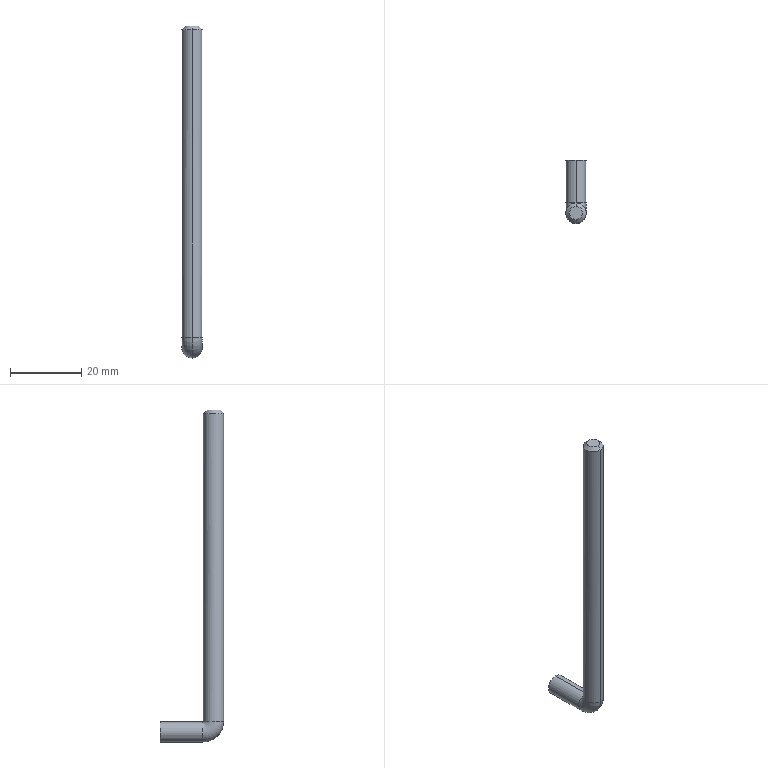Part | STEP file | RJWD-DY-0102_X2_5DE667DC95E8_37 | 1 solid | 10 faces | box 5.7 x 17.85 x 93.35 mm | volume 2651 mm3 | cylinder 4 | cone 2 | plane 2 | torus 2 | commonest cylinder face diameters 5.7 x4
STEP:
#1=CARTESIAN_POINT('',(0.,0.,0.));
#2=DIRECTION('',(0.,0.,1.));
#3=DIRECTION('',(1.,0.,0.));
#4=AXIS2_PLACEMENT_3D('',#1,#2,#3);
#5=CARTESIAN_POINT('',(-506.773,4247.223,1752.144));
#6=VERTEX_POINT('',#5);
#7=CARTESIAN_POINT('',(-503.923,4250.073,1752.144));
#8=VERTEX_POINT('',#7);
#9=CARTESIAN_POINT('',(-506.773,4250.073,1752.144));
#10=DIRECTION('',(0.,0.,1.));
#11=DIRECTION('',(0.,-1.,0.));
#12=AXIS2_PLACEMENT_3D('',#9,#10,#11);
#13=CIRCLE('',#12,2.85);
#14=CARTESIAN_POINT('',(-506.773,4250.073,1752.644));
#15=DIRECTION('',(0.,0.,-1.));
#16=DIRECTION('',(1.,0.,0.));
#17=AXIS2_PLACEMENT_3D('',#14,#15,#16);
#18=CONICAL_SURFACE('',#17,2.35,0.7854);
#19=CARTESIAN_POINT('',(1.571,0.5));
#20=DIRECTION('',(-1.,0.));
#21=VECTOR('',#20,1.);
#22=LINE('',#19,#21);
#23=(GEOMETRIC_REPRESENTATION_CONTEXT(2)PARAMETRIC_REPRESENTATION_CONTEXT()REPRESENTATION_CONTEXT('',''));
#24=DEFINITIONAL_REPRESENTATION('',(#22),#23);
#25=PCURVE('',#18,#24);
#26=CARTESIAN_POINT('',(-506.773,4250.073,1665.644));
#27=DIRECTION('',(0.,0.,1.));
#28=DIRECTION('',(0.,1.,0.));
#29=AXIS2_PLACEMENT_3D('',#26,#27,#28);
#30=CYLINDRICAL_SURFACE('',#29,2.85);
#31=CARTESIAN_POINT('',(3.142,86.5));
#32=DIRECTION('',(1.,0.));
#33=VECTOR('',#32,1.);
#34=LINE('',#31,#33);
#35=(GEOMETRIC_REPRESENTATION_CONTEXT(2)PARAMETRIC_REPRESENTATION_CONTEXT()REPRESENTATION_CONTEXT('',''));
#36=DEFINITIONAL_REPRESENTATION('',(#34),#35);
#37=PCURVE('',#30,#36);
#38=SURFACE_CURVE('',#13,(#25,#37),.PCURVE_S1.);
#39=EDGE_CURVE('',#6,#8,#38,.T.);
#40=ORIENTED_EDGE('',*,*,#39,.T.);
#41=CARTESIAN_POINT('',(-506.773,4252.923,1752.144));
#42=VERTEX_POINT('',#41);
#43=CARTESIAN_POINT('',(-506.773,4250.073,1752.144));
#44=DIRECTION('',(0.,0.,1.));
#45=DIRECTION('',(1.,0.,0.));
#46=AXIS2_PLACEMENT_3D('',#43,#44,#45);
#47=CIRCLE('',#46,2.85);
#48=CARTESIAN_POINT('',(0.,0.5));
#49=DIRECTION('',(-1.,0.));
#50=VECTOR('',#49,1.);
#51=LINE('',#48,#50);
#52=(GEOMETRIC_REPRESENTATION_CONTEXT(2)PARAMETRIC_REPRESENTATION_CONTEXT()REPRESENTATION_CONTEXT('',''));
#53=DEFINITIONAL_REPRESENTATION('',(#51),#52);
#54=PCURVE('',#18,#53);
#55=CARTESIAN_POINT('',(4.712,86.5));
#56=DIRECTION('',(1.,0.));
#57=VECTOR('',#56,1.);
#58=LINE('',#55,#57);
#59=(GEOMETRIC_REPRESENTATION_CONTEXT(2)PARAMETRIC_REPRESENTATION_CONTEXT()REPRESENTATION_CONTEXT('',''));
#60=DEFINITIONAL_REPRESENTATION('',(#58),#59);
#61=PCURVE('',#30,#60);
#62=SURFACE_CURVE('',#47,(#54,#61),.PCURVE_S1.);
#63=EDGE_CURVE('',#8,#42,#62,.T.);
#64=ORIENTED_EDGE('',*,*,#63,.T.);
#65=CARTESIAN_POINT('',(-506.773,4251.923,1753.144));
#66=VERTEX_POINT('',#65);
#67=CARTESIAN_POINT('',(-506.773,4251.923,1753.144));
#68=DIRECTION('',(0.,0.7071,-0.7071));
#69=VECTOR('',#68,1.);
#70=LINE('',#67,#69);
#71=CARTESIAN_POINT('',(-1.571,-0.5));
#72=DIRECTION('',(0.,1.));
#73=VECTOR('',#72,1.);
#74=LINE('',#71,#73);
#75=(GEOMETRIC_REPRESENTATION_CONTEXT(2)PARAMETRIC_REPRESENTATION_CONTEXT()REPRESENTATION_CONTEXT('',''));
#76=DEFINITIONAL_REPRESENTATION('',(#74),#75);
#77=PCURVE('',#18,#76);
#78=CARTESIAN_POINT('',(-506.773,4250.073,1752.644));
#79=DIRECTION('',(0.,0.,-1.));
#80=DIRECTION('',(1.,0.,0.));
#81=AXIS2_PLACEMENT_3D('',#78,#79,#80);
#82=CONICAL_SURFACE('',#81,2.35,0.7854);
#83=CARTESIAN_POINT('',(4.712,-0.5));
#84=DIRECTION('',(0.,1.));
#85=VECTOR('',#84,1.);
#86=LINE('',#83,#85);
#87=(GEOMETRIC_REPRESENTATION_CONTEXT(2)PARAMETRIC_REPRESENTATION_CONTEXT()REPRESENTATION_CONTEXT('',''));
#88=DEFINITIONAL_REPRESENTATION('',(#86),#87);
#89=PCURVE('',#82,#88);
#90=SURFACE_CURVE('',#70,(#77,#89),.PCURVE_S1.);
#91=EDGE_CURVE('',#66,#42,#90,.T.);
#92=ORIENTED_EDGE('',*,*,#91,.F.);
#93=CARTESIAN_POINT('',(-504.923,4250.073,1753.144));
#94=VERTEX_POINT('',#93);
#95=CARTESIAN_POINT('',(-506.773,4250.073,1753.144));
#96=DIRECTION('',(0.,0.,1.));
#97=DIRECTION('',(1.,0.,0.));
#98=AXIS2_PLACEMENT_3D('',#95,#96,#97);
#99=CIRCLE('',#98,1.85);
#100=CARTESIAN_POINT('',(0.,-0.5));
#101=DIRECTION('',(-1.,0.));
#102=VECTOR('',#101,1.);
#103=LINE('',#100,#102);
#104=(GEOMETRIC_REPRESENTATION_CONTEXT(2)PARAMETRIC_REPRESENTATION_CONTEXT()REPRESENTATION_CONTEXT('',''));
#105=DEFINITIONAL_REPRESENTATION('',(#103),#104);
#106=PCURVE('',#18,#105);
#107=CARTESIAN_POINT('',(-506.773,4250.073,1753.144));
#108=DIRECTION('',(0.,0.,1.));
#109=DIRECTION('',(0.,1.,0.));
#110=AXIS2_PLACEMENT_3D('',#107,#108,#109);
#111=PLANE('',#110);
#112=CARTESIAN_POINT('',(0.,0.));
#113=DIRECTION('',(0.,-1.));
#114=AXIS2_PLACEMENT_2D('',#112,#113);
#115=CIRCLE('',#114,1.85);
#116=(GEOMETRIC_REPRESENTATION_CONTEXT(2)PARAMETRIC_REPRESENTATION_CONTEXT()REPRESENTATION_CONTEXT('',''));
#117=DEFINITIONAL_REPRESENTATION('',(#115),#116);
#118=PCURVE('',#111,#117);
#119=SURFACE_CURVE('',#99,(#106,#118),.PCURVE_S1.);
#120=EDGE_CURVE('',#94,#66,#119,.T.);
#121=ORIENTED_EDGE('',*,*,#120,.F.);
#122=CARTESIAN_POINT('',(-506.773,4248.223,1753.144));
#123=VERTEX_POINT('',#122);
#124=CARTESIAN_POINT('',(-506.773,4250.073,1753.144));
#125=DIRECTION('',(0.,0.,1.));
#126=DIRECTION('',(0.,-1.,0.));
#127=AXIS2_PLACEMENT_3D('',#124,#125,#126);
#128=CIRCLE('',#127,1.85);
#129=CARTESIAN_POINT('',(1.571,-0.5));
#130=DIRECTION('',(-1.,0.));
#131=VECTOR('',#130,1.);
#132=LINE('',#129,#131);
#133=(GEOMETRIC_REPRESENTATION_CONTEXT(2)PARAMETRIC_REPRESENTATION_CONTEXT()REPRESENTATION_CONTEXT('',''));
#134=DEFINITIONAL_REPRESENTATION('',(#132),#133);
#135=PCURVE('',#18,#134);
#136=CARTESIAN_POINT('',(0.,0.));
#137=DIRECTION('',(-1.,0.));
#138=AXIS2_PLACEMENT_2D('',#136,#137);
#139=CIRCLE('',#138,1.85);
#140=(GEOMETRIC_REPRESENTATION_CONTEXT(2)PARAMETRIC_REPRESENTATION_CONTEXT()REPRESENTATION_CONTEXT('',''));
#141=DEFINITIONAL_REPRESENTATION('',(#139),#140);
#142=PCURVE('',#111,#141);
#143=SURFACE_CURVE('',#128,(#135,#142),.PCURVE_S1.);
#144=EDGE_CURVE('',#123,#94,#143,.T.);
#145=ORIENTED_EDGE('',*,*,#144,.F.);
#146=CARTESIAN_POINT('',(-506.773,4248.223,1753.144));
#147=DIRECTION('',(0.,-0.7071,-0.7071));
#148=VECTOR('',#147,1.);
#149=LINE('',#146,#148);
#150=CARTESIAN_POINT('',(1.571,-0.5));
#151=DIRECTION('',(0.,1.));
#152=VECTOR('',#151,1.);
#153=LINE('',#150,#152);
#154=(GEOMETRIC_REPRESENTATION_CONTEXT(2)PARAMETRIC_REPRESENTATION_CONTEXT()REPRESENTATION_CONTEXT('',''));
#155=DEFINITIONAL_REPRESENTATION('',(#153),#154);
#156=PCURVE('',#18,#155);
#157=CARTESIAN_POINT('',(1.571,-0.5));
#158=DIRECTION('',(0.,1.));
#159=VECTOR('',#158,1.);
#160=LINE('',#157,#159);
#161=(GEOMETRIC_REPRESENTATION_CONTEXT(2)PARAMETRIC_REPRESENTATION_CONTEXT()REPRESENTATION_CONTEXT('',''));
#162=DEFINITIONAL_REPRESENTATION('',(#160),#161);
#163=PCURVE('',#82,#162);
#164=SURFACE_CURVE('',#149,(#156,#163),.PCURVE_S1.);
#165=EDGE_CURVE('',#123,#6,#164,.T.);
#166=ORIENTED_EDGE('',*,*,#165,.T.);
#167=EDGE_LOOP('',(#40,#64,#92,#121,#145,#166));
#168=FACE_BOUND('',#167,.T.);
#169=ADVANCED_FACE('',(#168),#18,.T.);
#170=CARTESIAN_POINT('',(-509.623,4250.073,1752.144));
#171=VERTEX_POINT('',#170);
#172=CARTESIAN_POINT('',(-506.773,4250.073,1752.144));
#173=DIRECTION('',(0.,0.,1.));
#174=DIRECTION('',(0.,1.,0.));
#175=AXIS2_PLACEMENT_3D('',#172,#173,#174);
#176=CIRCLE('',#175,2.85);
#177=CARTESIAN_POINT('',(4.712,0.5));
#178=DIRECTION('',(-1.,0.));
#179=VECTOR('',#178,1.);
#180=LINE('',#177,#179);
#181=(GEOMETRIC_REPRESENTATION_CONTEXT(2)PARAMETRIC_REPRESENTATION_CONTEXT()REPRESENTATION_CONTEXT('',''));
#182=DEFINITIONAL_REPRESENTATION('',(#180),#181);
#183=PCURVE('',#82,#182);
#184=CARTESIAN_POINT('',(-506.773,4250.073,1665.644));
#185=DIRECTION('',(0.,0.,1.));
#186=DIRECTION('',(0.,1.,0.));
#187=AXIS2_PLACEMENT_3D('',#184,#185,#186);
#188=CYLINDRICAL_SURFACE('',#187,2.85);
#189=CARTESIAN_POINT('',(0.,86.5));
#190=DIRECTION('',(1.,0.));
#191=VECTOR('',#190,1.);
#192=LINE('',#189,#191);
#193=(GEOMETRIC_REPRESENTATION_CONTEXT(2)PARAMETRIC_REPRESENTATION_CONTEXT()REPRESENTATION_CONTEXT('',''));
#194=DEFINITIONAL_REPRESENTATION('',(#192),#193);
#195=PCURVE('',#188,#194);
#196=SURFACE_CURVE('',#176,(#183,#195),.PCURVE_S1.);
#197=EDGE_CURVE('',#42,#171,#196,.T.);
#198=ORIENTED_EDGE('',*,*,#197,.T.);
#199=CARTESIAN_POINT('',(-506.773,4250.073,1752.144));
#200=DIRECTION('',(0.,0.,1.));
#201=DIRECTION('',(-1.,0.,0.));
#202=AXIS2_PLACEMENT_3D('',#199,#200,#201);
#203=CIRCLE('',#202,2.85);
#204=CARTESIAN_POINT('',(3.142,0.5));
#205=DIRECTION('',(-1.,0.));
#206=VECTOR('',#205,1.);
#207=LINE('',#204,#206);
#208=(GEOMETRIC_REPRESENTATION_CONTEXT(2)PARAMETRIC_REPRESENTATION_CONTEXT()REPRESENTATION_CONTEXT('',''));
#209=DEFINITIONAL_REPRESENTATION('',(#207),#208);
#210=PCURVE('',#82,#209);
#211=CARTESIAN_POINT('',(1.571,86.5));
#212=DIRECTION('',(1.,0.));
#213=VECTOR('',#212,1.);
#214=LINE('',#211,#213);
#215=(GEOMETRIC_REPRESENTATION_CONTEXT(2)PARAMETRIC_REPRESENTATION_CONTEXT()REPRESENTATION_CONTEXT('',''));
#216=DEFINITIONAL_REPRESENTATION('',(#214),#215);
#217=PCURVE('',#188,#216);
#218=SURFACE_CURVE('',#203,(#210,#217),.PCURVE_S1.);
#219=EDGE_CURVE('',#171,#6,#218,.T.);
#220=ORIENTED_EDGE('',*,*,#219,.T.);
#221=ORIENTED_EDGE('',*,*,#165,.F.);
#222=CARTESIAN_POINT('',(-508.623,4250.073,1753.144));
#223=VERTEX_POINT('',#222);
#224=CARTESIAN_POINT('',(-506.773,4250.073,1753.144));
#225=DIRECTION('',(0.,0.,1.));
#226=DIRECTION('',(-1.,0.,0.));
#227=AXIS2_PLACEMENT_3D('',#224,#225,#226);
#228=CIRCLE('',#227,1.85);
#229=CARTESIAN_POINT('',(3.142,-0.5));
#230=DIRECTION('',(-1.,0.));
#231=VECTOR('',#230,1.);
#232=LINE('',#229,#231);
#233=(GEOMETRIC_REPRESENTATION_CONTEXT(2)PARAMETRIC_REPRESENTATION_CONTEXT()REPRESENTATION_CONTEXT('',''));
#234=DEFINITIONAL_REPRESENTATION('',(#232),#233);
#235=PCURVE('',#82,#234);
#236=CARTESIAN_POINT('',(0.,0.));
#237=DIRECTION('',(0.,1.));
#238=AXIS2_PLACEMENT_2D('',#236,#237);
#239=CIRCLE('',#238,1.85);
#240=(GEOMETRIC_REPRESENTATION_CONTEXT(2)PARAMETRIC_REPRESENTATION_CONTEXT()REPRESENTATION_CONTEXT('',''));
#241=DEFINITIONAL_REPRESENTATION('',(#239),#240);
#242=PCURVE('',#111,#241);
#243=SURFACE_CURVE('',#228,(#235,#242),.PCURVE_S1.);
#244=EDGE_CURVE('',#223,#123,#243,.T.);
#245=ORIENTED_EDGE('',*,*,#244,.F.);
#246=CARTESIAN_POINT('',(-506.773,4250.073,1753.144));
#247=DIRECTION('',(0.,0.,1.));
#248=DIRECTION('',(0.,1.,0.));
#249=AXIS2_PLACEMENT_3D('',#246,#247,#248);
#250=CIRCLE('',#249,1.85);
#251=CARTESIAN_POINT('',(4.712,-0.5));
#252=DIRECTION('',(-1.,0.));
#253=VECTOR('',#252,1.);
#254=LINE('',#251,#253);
#255=(GEOMETRIC_REPRESENTATION_CONTEXT(2)PARAMETRIC_REPRESENTATION_CONTEXT()REPRESENTATION_CONTEXT('',''));
#256=DEFINITIONAL_REPRESENTATION('',(#254),#255);
#257=PCURVE('',#82,#256);
#258=CARTESIAN_POINT('',(0.,0.));
#259=DIRECTION('',(1.,0.));
#260=AXIS2_PLACEMENT_2D('',#258,#259);
#261=CIRCLE('',#260,1.85);
#262=(GEOMETRIC_REPRESENTATION_CONTEXT(2)PARAMETRIC_REPRESENTATION_CONTEXT()REPRESENTATION_CONTEXT('',''));
#263=DEFINITIONAL_REPRESENTATION('',(#261),#262);
#264=PCURVE('',#111,#263);
#265=SURFACE_CURVE('',#250,(#257,#264),.PCURVE_S1.);
#266=EDGE_CURVE('',#66,#223,#265,.T.);
#267=ORIENTED_EDGE('',*,*,#266,.F.);
#268=ORIENTED_EDGE('',*,*,#91,.T.);
#269=EDGE_LOOP('',(#198,#220,#221,#245,#267,#268));
#270=FACE_BOUND('',#269,.T.);
#271=ADVANCED_FACE('',(#270),#82,.T.);
#272=ORIENTED_EDGE('',*,*,#144,.F.);
#273=ORIENTED_EDGE('',*,*,#244,.F.);
#274=ORIENTED_EDGE('',*,*,#266,.F.);
#275=ORIENTED_EDGE('',*,*,#120,.F.);
#276=EDGE_LOOP('',(#272,#273,#274,#275));
#277=FACE_BOUND('',#276,.F.);
#278=ADVANCED_FACE('',(#277),#111,.T.);
#279=CARTESIAN_POINT('',(-506.773,4247.223,1665.644));
#280=VERTEX_POINT('',#279);
#281=CARTESIAN_POINT('',(-506.773,4252.923,1665.644));
#282=VERTEX_POINT('',#281);
#283=CARTESIAN_POINT('',(-506.773,4250.073,1665.644));
#284=DIRECTION('',(0.,0.,-1.));
#285=DIRECTION('',(0.,-1.,0.));
#286=AXIS2_PLACEMENT_3D('',#283,#284,#285);
#287=CIRCLE('',#286,2.85);
#288=CARTESIAN_POINT('',(3.142,0.));
#289=DIRECTION('',(-1.,0.));
#290=VECTOR('',#289,1.);
#291=LINE('',#288,#290);
#292=(GEOMETRIC_REPRESENTATION_CONTEXT(2)PARAMETRIC_REPRESENTATION_CONTEXT()REPRESENTATION_CONTEXT('',''));
#293=DEFINITIONAL_REPRESENTATION('',(#291),#292);
#294=PCURVE('',#188,#293);
#295=CARTESIAN_POINT('',(-506.773,4253.073,1665.644));
#296=DIRECTION('',(-1.,0.,0.));
#297=DIRECTION('',(0.,0.,-1.));
#298=AXIS2_PLACEMENT_3D('',#295,#296,#297);
#299=TOROIDAL_SURFACE('',#298,3.,2.85);
#300=CARTESIAN_POINT('',(1.571,0.));
#301=DIRECTION('',(0.,1.));
#302=VECTOR('',#301,1.);
#303=LINE('',#300,#302);
#304=(GEOMETRIC_REPRESENTATION_CONTEXT(2)PARAMETRIC_REPRESENTATION_CONTEXT()REPRESENTATION_CONTEXT('',''));
#305=DEFINITIONAL_REPRESENTATION('',(#303),#304);
#306=PCURVE('',#299,#305);
#307=SURFACE_CURVE('',#287,(#294,#306),.PCURVE_S1.);
#308=EDGE_CURVE('',#280,#282,#307,.T.);
#309=ORIENTED_EDGE('',*,*,#308,.F.);
#310=CARTESIAN_POINT('',(-506.773,4247.223,1665.644));
#311=DIRECTION('',(0.,0.,1.));
#312=VECTOR('',#311,1.);
#313=LINE('',#310,#312);
#314=CARTESIAN_POINT('',(3.142,0.));
#315=DIRECTION('',(0.,1.));
#316=VECTOR('',#315,1.);
#317=LINE('',#314,#316);
#318=(GEOMETRIC_REPRESENTATION_CONTEXT(2)PARAMETRIC_REPRESENTATION_CONTEXT()REPRESENTATION_CONTEXT('',''));
#319=DEFINITIONAL_REPRESENTATION('',(#317),#318);
#320=PCURVE('',#188,#319);
#321=CARTESIAN_POINT('',(3.142,0.));
#322=DIRECTION('',(0.,1.));
#323=VECTOR('',#322,1.);
#324=LINE('',#321,#323);
#325=(GEOMETRIC_REPRESENTATION_CONTEXT(2)PARAMETRIC_REPRESENTATION_CONTEXT()REPRESENTATION_CONTEXT('',''));
#326=DEFINITIONAL_REPRESENTATION('',(#324),#325);
#327=PCURVE('',#30,#326);
#328=SURFACE_CURVE('',#313,(#320,#327),.PCURVE_S1.);
#329=EDGE_CURVE('',#280,#6,#328,.T.);
#330=ORIENTED_EDGE('',*,*,#329,.T.);
#331=ORIENTED_EDGE('',*,*,#219,.F.);
#332=ORIENTED_EDGE('',*,*,#197,.F.);
#333=CARTESIAN_POINT('',(-506.773,4252.923,1665.644));
#334=DIRECTION('',(0.,0.,1.));
#335=VECTOR('',#334,1.);
#336=LINE('',#333,#335);
#337=CARTESIAN_POINT('',(0.,0.));
#338=DIRECTION('',(0.,1.));
#339=VECTOR('',#338,1.);
#340=LINE('',#337,#339);
#341=(GEOMETRIC_REPRESENTATION_CONTEXT(2)PARAMETRIC_REPRESENTATION_CONTEXT()REPRESENTATION_CONTEXT('',''));
#342=DEFINITIONAL_REPRESENTATION('',(#340),#341);
#343=PCURVE('',#188,#342);
#344=CARTESIAN_POINT('',(6.283,0.));
#345=DIRECTION('',(0.,1.));
#346=VECTOR('',#345,1.);
#347=LINE('',#344,#346);
#348=(GEOMETRIC_REPRESENTATION_CONTEXT(2)PARAMETRIC_REPRESENTATION_CONTEXT()REPRESENTATION_CONTEXT('',''));
#349=DEFINITIONAL_REPRESENTATION('',(#347),#348);
#350=PCURVE('',#30,#349);
#351=SURFACE_CURVE('',#336,(#343,#350),.PCURVE_S1.);
#352=EDGE_CURVE('',#282,#42,#351,.T.);
#353=ORIENTED_EDGE('',*,*,#352,.F.);
#354=EDGE_LOOP('',(#309,#330,#331,#332,#353));
#355=FACE_BOUND('',#354,.T.);
#356=ADVANCED_FACE('',(#355),#188,.T.);
#357=CARTESIAN_POINT('',(-506.773,4250.073,1665.644));
#358=DIRECTION('',(0.,0.,-1.));
#359=DIRECTION('',(0.,1.,0.));
#360=AXIS2_PLACEMENT_3D('',#357,#358,#359);
#361=CIRCLE('',#360,2.85);
#362=CARTESIAN_POINT('',(6.283,0.));
#363=DIRECTION('',(-1.,0.));
#364=VECTOR('',#363,1.);
#365=LINE('',#362,#364);
#366=(GEOMETRIC_REPRESENTATION_CONTEXT(2)PARAMETRIC_REPRESENTATION_CONTEXT()REPRESENTATION_CONTEXT('',''));
#367=DEFINITIONAL_REPRESENTATION('',(#365),#366);
#368=PCURVE('',#30,#367);
#369=CARTESIAN_POINT('',(-506.773,4253.073,1665.644));
#370=DIRECTION('',(-1.,0.,0.));
#371=DIRECTION('',(0.,0.,-1.));
#372=AXIS2_PLACEMENT_3D('',#369,#370,#371);
#373=TOROIDAL_SURFACE('',#372,3.,2.85);
#374=CARTESIAN_POINT('',(1.571,3.142));
#375=DIRECTION('',(0.,1.));
#376=VECTOR('',#375,1.);
#377=LINE('',#374,#376);
#378=(GEOMETRIC_REPRESENTATION_CONTEXT(2)PARAMETRIC_REPRESENTATION_CONTEXT()REPRESENTATION_CONTEXT('',''));
#379=DEFINITIONAL_REPRESENTATION('',(#377),#378);
#380=PCURVE('',#373,#379);
#381=SURFACE_CURVE('',#361,(#368,#380),.PCURVE_S1.);
#382=EDGE_CURVE('',#282,#280,#381,.T.);
#383=ORIENTED_EDGE('',*,*,#382,.F.);
#384=ORIENTED_EDGE('',*,*,#352,.T.);
#385=ORIENTED_EDGE('',*,*,#63,.F.);
#386=ORIENTED_EDGE('',*,*,#39,.F.);
#387=ORIENTED_EDGE('',*,*,#329,.F.);
#388=EDGE_LOOP('',(#383,#384,#385,#386,#387));
#389=FACE_BOUND('',#388,.T.);
#390=ADVANCED_FACE('',(#389),#30,.T.);
#391=ORIENTED_EDGE('',*,*,#382,.T.);
#392=CARTESIAN_POINT('',(-506.773,4253.073,1659.794));
#393=VERTEX_POINT('',#392);
#394=CARTESIAN_POINT('',(-506.773,4253.073,1665.644));
#395=DIRECTION('',(-1.,0.,0.));
#396=DIRECTION('',(0.,0.,-1.));
#397=AXIS2_PLACEMENT_3D('',#394,#395,#396);
#398=CIRCLE('',#397,5.85);
#399=CARTESIAN_POINT('',(0.,6.283));
#400=DIRECTION('',(1.,0.));
#401=VECTOR('',#400,1.);
#402=LINE('',#399,#401);
#403=(GEOMETRIC_REPRESENTATION_CONTEXT(2)PARAMETRIC_REPRESENTATION_CONTEXT()REPRESENTATION_CONTEXT('',''));
#404=DEFINITIONAL_REPRESENTATION('',(#402),#403);
#405=PCURVE('',#373,#404);
#406=CARTESIAN_POINT('',(0.,0.));
#407=DIRECTION('',(1.,0.));
#408=VECTOR('',#407,1.);
#409=LINE('',#406,#408);
#410=(GEOMETRIC_REPRESENTATION_CONTEXT(2)PARAMETRIC_REPRESENTATION_CONTEXT()REPRESENTATION_CONTEXT('',''));
#411=DEFINITIONAL_REPRESENTATION('',(#409),#410);
#412=PCURVE('',#299,#411);
#413=SURFACE_CURVE('',#398,(#405,#412),.PCURVE_S1.);
#414=EDGE_CURVE('',#393,#280,#413,.T.);
#415=ORIENTED_EDGE('',*,*,#414,.F.);
#416=CARTESIAN_POINT('',(-506.773,4253.073,1665.494));
#417=VERTEX_POINT('',#416);
#418=CARTESIAN_POINT('',(-506.773,4253.073,1662.644));
#419=DIRECTION('',(0.,-1.,0.));
#420=DIRECTION('',(0.,0.,-1.));
#421=AXIS2_PLACEMENT_3D('',#418,#419,#420);
#422=CIRCLE('',#421,2.85);
#423=CARTESIAN_POINT('',(0.,6.283));
#424=DIRECTION('',(0.,-1.));
#425=VECTOR('',#424,1.);
#426=LINE('',#423,#425);
#427=(GEOMETRIC_REPRESENTATION_CONTEXT(2)PARAMETRIC_REPRESENTATION_CONTEXT()REPRESENTATION_CONTEXT('',''));
#428=DEFINITIONAL_REPRESENTATION('',(#426),#427);
#429=PCURVE('',#373,#428);
#430=CARTESIAN_POINT('',(-506.773,4265.073,1662.644));
#431=DIRECTION('',(0.,-1.,0.));
#432=DIRECTION('',(0.,0.,1.));
#433=AXIS2_PLACEMENT_3D('',#430,#431,#432);
#434=CYLINDRICAL_SURFACE('',#433,2.85);
#435=CARTESIAN_POINT('',(3.142,12.));
#436=DIRECTION('',(1.,0.));
#437=VECTOR('',#436,1.);
#438=LINE('',#435,#437);
#439=(GEOMETRIC_REPRESENTATION_CONTEXT(2)PARAMETRIC_REPRESENTATION_CONTEXT()REPRESENTATION_CONTEXT('',''));
#440=DEFINITIONAL_REPRESENTATION('',(#438),#439);
#441=PCURVE('',#434,#440);
#442=SURFACE_CURVE('',#422,(#429,#441),.PCURVE_S1.);
#443=EDGE_CURVE('',#393,#417,#442,.T.);
#444=ORIENTED_EDGE('',*,*,#443,.T.);
#445=CARTESIAN_POINT('',(-506.773,4253.073,1665.644));
#446=DIRECTION('',(-1.,0.,0.));
#447=DIRECTION('',(0.,0.,-1.));
#448=AXIS2_PLACEMENT_3D('',#445,#446,#447);
#449=CIRCLE('',#448,0.15);
#450=CARTESIAN_POINT('',(0.,3.142));
#451=DIRECTION('',(1.,0.));
#452=VECTOR('',#451,1.);
#453=LINE('',#450,#452);
#454=(GEOMETRIC_REPRESENTATION_CONTEXT(2)PARAMETRIC_REPRESENTATION_CONTEXT()REPRESENTATION_CONTEXT('',''));
#455=DEFINITIONAL_REPRESENTATION('',(#453),#454);
#456=PCURVE('',#373,#455);
#457=CARTESIAN_POINT('',(0.,3.142));
#458=DIRECTION('',(1.,0.));
#459=VECTOR('',#458,1.);
#460=LINE('',#457,#459);
#461=(GEOMETRIC_REPRESENTATION_CONTEXT(2)PARAMETRIC_REPRESENTATION_CONTEXT()REPRESENTATION_CONTEXT('',''));
#462=DEFINITIONAL_REPRESENTATION('',(#460),#461);
#463=PCURVE('',#299,#462);
#464=SURFACE_CURVE('',#449,(#456,#463),.PCURVE_S1.);
#465=EDGE_CURVE('',#417,#282,#464,.T.);
#466=ORIENTED_EDGE('',*,*,#465,.T.);
#467=EDGE_LOOP('',(#391,#415,#444,#466));
#468=FACE_BOUND('',#467,.T.);
#469=ADVANCED_FACE('',(#468),#373,.T.);
#470=ORIENTED_EDGE('',*,*,#308,.T.);
#471=ORIENTED_EDGE('',*,*,#465,.F.);
#472=CARTESIAN_POINT('',(-506.773,4253.073,1662.644));
#473=DIRECTION('',(0.,-1.,0.));
#474=DIRECTION('',(0.,0.,1.));
#475=AXIS2_PLACEMENT_3D('',#472,#473,#474);
#476=CIRCLE('',#475,2.85);
#477=CARTESIAN_POINT('',(0.,3.142));
#478=DIRECTION('',(0.,-1.));
#479=VECTOR('',#478,1.);
#480=LINE('',#477,#479);
#481=(GEOMETRIC_REPRESENTATION_CONTEXT(2)PARAMETRIC_REPRESENTATION_CONTEXT()REPRESENTATION_CONTEXT('',''));
#482=DEFINITIONAL_REPRESENTATION('',(#480),#481);
#483=PCURVE('',#299,#482);
#484=CARTESIAN_POINT('',(-506.773,4265.073,1662.644));
#485=DIRECTION('',(0.,-1.,0.));
#486=DIRECTION('',(0.,0.,1.));
#487=AXIS2_PLACEMENT_3D('',#484,#485,#486);
#488=CYLINDRICAL_SURFACE('',#487,2.85);
#489=CARTESIAN_POINT('',(0.,12.));
#490=DIRECTION('',(1.,0.));
#491=VECTOR('',#490,1.);
#492=LINE('',#489,#491);
#493=(GEOMETRIC_REPRESENTATION_CONTEXT(2)PARAMETRIC_REPRESENTATION_CONTEXT()REPRESENTATION_CONTEXT('',''));
#494=DEFINITIONAL_REPRESENTATION('',(#492),#493);
#495=PCURVE('',#488,#494);
#496=SURFACE_CURVE('',#476,(#483,#495),.PCURVE_S1.);
#497=EDGE_CURVE('',#417,#393,#496,.T.);
#498=ORIENTED_EDGE('',*,*,#497,.T.);
#499=ORIENTED_EDGE('',*,*,#414,.T.);
#500=EDGE_LOOP('',(#470,#471,#498,#499));
#501=FACE_BOUND('',#500,.T.);
#502=ADVANCED_FACE('',(#501),#299,.T.);
#503=ORIENTED_EDGE('',*,*,#497,.F.);
#504=CARTESIAN_POINT('',(-506.773,4265.073,1665.494));
#505=VERTEX_POINT('',#504);
#506=CARTESIAN_POINT('',(-506.773,4253.073,1665.494));
#507=DIRECTION('',(0.,1.,0.));
#508=VECTOR('',#507,1.);
#509=LINE('',#506,#508);
#510=CARTESIAN_POINT('',(0.,12.));
#511=DIRECTION('',(0.,-1.));
#512=VECTOR('',#511,1.);
#513=LINE('',#510,#512);
#514=(GEOMETRIC_REPRESENTATION_CONTEXT(2)PARAMETRIC_REPRESENTATION_CONTEXT()REPRESENTATION_CONTEXT('',''));
#515=DEFINITIONAL_REPRESENTATION('',(#513),#514);
#516=PCURVE('',#488,#515);
#517=CARTESIAN_POINT('',(6.283,12.));
#518=DIRECTION('',(0.,-1.));
#519=VECTOR('',#518,1.);
#520=LINE('',#517,#519);
#521=(GEOMETRIC_REPRESENTATION_CONTEXT(2)PARAMETRIC_REPRESENTATION_CONTEXT()REPRESENTATION_CONTEXT('',''));
#522=DEFINITIONAL_REPRESENTATION('',(#520),#521);
#523=PCURVE('',#434,#522);
#524=SURFACE_CURVE('',#509,(#516,#523),.PCURVE_S1.);
#525=EDGE_CURVE('',#417,#505,#524,.T.);
#526=ORIENTED_EDGE('',*,*,#525,.T.);
#527=CARTESIAN_POINT('',(-506.773,4265.073,1659.794));
#528=VERTEX_POINT('',#527);
#529=CARTESIAN_POINT('',(-506.773,4265.073,1662.644));
#530=DIRECTION('',(0.,1.,0.));
#531=DIRECTION('',(0.,0.,-1.));
#532=AXIS2_PLACEMENT_3D('',#529,#530,#531);
#533=CIRCLE('',#532,2.85);
#534=CARTESIAN_POINT('',(3.142,0.));
#535=DIRECTION('',(-1.,0.));
#536=VECTOR('',#535,1.);
#537=LINE('',#534,#536);
#538=(GEOMETRIC_REPRESENTATION_CONTEXT(2)PARAMETRIC_REPRESENTATION_CONTEXT()REPRESENTATION_CONTEXT('',''));
#539=DEFINITIONAL_REPRESENTATION('',(#537),#538);
#540=PCURVE('',#488,#539);
#541=CARTESIAN_POINT('',(-506.773,4265.073,1662.644));
#542=DIRECTION('',(0.,-1.,0.));
#543=DIRECTION('',(0.,0.,1.));
#544=AXIS2_PLACEMENT_3D('',#541,#542,#543);
#545=PLANE('',#544);
#546=CARTESIAN_POINT('',(-2.85,0.));
#547=CARTESIAN_POINT('',(-2.85,4.936));
#548=CARTESIAN_POINT('',(1.425,2.468));
#549=CARTESIAN_POINT('',(5.7,0.));
#550=CARTESIAN_POINT('',(1.425,-2.468));
#551=CARTESIAN_POINT('',(-2.85,-4.936));
#552=CARTESIAN_POINT('',(-2.85,0.));
#553=(BOUNDED_CURVE()B_SPLINE_CURVE(2,(#546,#547,#548,#549,#550,#551,#552),.UNSPECIFIED.,.T.,.F.)B_SPLINE_CURVE_WITH_KNOTS((1,2,2,2,2,1),(-2.094,0.,2.094,4.189,6.283,8.378),.UNSPECIFIED.)CURVE()GEOMETRIC_REPRESENTATION_ITEM()RATIONAL_B_SPLINE_CURVE((1.,0.5,1.,0.5,1.,0.5,1.))REPRESENTATION_ITEM(''));
#554=(GEOMETRIC_REPRESENTATION_CONTEXT(2)PARAMETRIC_REPRESENTATION_CONTEXT()REPRESENTATION_CONTEXT('',''));
#555=DEFINITIONAL_REPRESENTATION('',(#553),#554);
#556=PCURVE('',#545,#555);
#557=SURFACE_CURVE('',#533,(#540,#556),.PCURVE_S1.);
#558=EDGE_CURVE('',#528,#505,#557,.T.);
#559=ORIENTED_EDGE('',*,*,#558,.F.);
#560=CARTESIAN_POINT('',(-506.773,4253.073,1659.794));
#561=DIRECTION('',(0.,1.,0.));
#562=VECTOR('',#561,1.);
#563=LINE('',#560,#562);
#564=CARTESIAN_POINT('',(3.142,12.));
#565=DIRECTION('',(0.,-1.));
#566=VECTOR('',#565,1.);
#567=LINE('',#564,#566);
#568=(GEOMETRIC_REPRESENTATION_CONTEXT(2)PARAMETRIC_REPRESENTATION_CONTEXT()REPRESENTATION_CONTEXT('',''));
#569=DEFINITIONAL_REPRESENTATION('',(#567),#568);
#570=PCURVE('',#488,#569);
#571=CARTESIAN_POINT('',(3.142,12.));
#572=DIRECTION('',(0.,-1.));
#573=VECTOR('',#572,1.);
#574=LINE('',#571,#573);
#575=(GEOMETRIC_REPRESENTATION_CONTEXT(2)PARAMETRIC_REPRESENTATION_CONTEXT()REPRESENTATION_CONTEXT('',''));
#576=DEFINITIONAL_REPRESENTATION('',(#574),#575);
#577=PCURVE('',#434,#576);
#578=SURFACE_CURVE('',#563,(#570,#577),.PCURVE_S1.);
#579=EDGE_CURVE('',#393,#528,#578,.T.);
#580=ORIENTED_EDGE('',*,*,#579,.F.);
#581=EDGE_LOOP('',(#503,#526,#559,#580));
#582=FACE_BOUND('',#581,.T.);
#583=ADVANCED_FACE('',(#582),#488,.T.);
#584=ORIENTED_EDGE('',*,*,#443,.F.);
#585=ORIENTED_EDGE('',*,*,#579,.T.);
#586=CARTESIAN_POINT('',(-506.773,4265.073,1662.644));
#587=DIRECTION('',(0.,1.,0.));
#588=DIRECTION('',(0.,0.,1.));
#589=AXIS2_PLACEMENT_3D('',#586,#587,#588);
#590=CIRCLE('',#589,2.85);
#591=CARTESIAN_POINT('',(6.283,0.));
#592=DIRECTION('',(-1.,0.));
#593=VECTOR('',#592,1.);
#594=LINE('',#591,#593);
#595=(GEOMETRIC_REPRESENTATION_CONTEXT(2)PARAMETRIC_REPRESENTATION_CONTEXT()REPRESENTATION_CONTEXT('',''));
#596=DEFINITIONAL_REPRESENTATION('',(#594),#595);
#597=PCURVE('',#434,#596);
#598=CARTESIAN_POINT('',(2.85,0.));
#599=CARTESIAN_POINT('',(2.85,-4.936));
#600=CARTESIAN_POINT('',(-1.425,-2.468));
#601=CARTESIAN_POINT('',(-5.7,0.));
#602=CARTESIAN_POINT('',(-1.425,2.468));
#603=CARTESIAN_POINT('',(2.85,4.936));
#604=CARTESIAN_POINT('',(2.85,0.));
#605=(BOUNDED_CURVE()B_SPLINE_CURVE(2,(#598,#599,#600,#601,#602,#603,#604),.UNSPECIFIED.,.T.,.F.)B_SPLINE_CURVE_WITH_KNOTS((1,2,2,2,2,1),(-2.094,0.,2.094,4.189,6.283,8.378),.UNSPECIFIED.)CURVE()GEOMETRIC_REPRESENTATION_ITEM()RATIONAL_B_SPLINE_CURVE((1.,0.5,1.,0.5,1.,0.5,1.))REPRESENTATION_ITEM(''));
#606=(GEOMETRIC_REPRESENTATION_CONTEXT(2)PARAMETRIC_REPRESENTATION_CONTEXT()REPRESENTATION_CONTEXT('',''));
#607=DEFINITIONAL_REPRESENTATION('',(#605),#606);
#608=PCURVE('',#545,#607);
#609=SURFACE_CURVE('',#590,(#597,#608),.PCURVE_S1.);
#610=EDGE_CURVE('',#505,#528,#609,.T.);
#611=ORIENTED_EDGE('',*,*,#610,.F.);
#612=ORIENTED_EDGE('',*,*,#525,.F.);
#613=EDGE_LOOP('',(#584,#585,#611,#612));
#614=FACE_BOUND('',#613,.T.);
#615=ADVANCED_FACE('',(#614),#434,.T.);
#616=ORIENTED_EDGE('',*,*,#558,.F.);
#617=ORIENTED_EDGE('',*,*,#610,.F.);
#618=EDGE_LOOP('',(#616,#617));
#619=FACE_BOUND('',#618,.F.);
#620=ADVANCED_FACE('',(#619),#545,.F.);
#621=CLOSED_SHELL('',(#169,#271,#278,#356,#390,#469,#502,#583,#615,#620));
#622=MANIFOLD_SOLID_BREP('',#621);
#623=(LENGTH_UNIT()NAMED_UNIT(*)SI_UNIT(.MILLI.,.METRE.));
#624=UNCERTAINTY_MEASURE_WITH_UNIT(LENGTH_MEASURE(0.0000001),#623,'','');
#625=(NAMED_UNIT(*)PLANE_ANGLE_UNIT()SI_UNIT($,.RADIAN.));
#626=(NAMED_UNIT(*)SI_UNIT($,.STERADIAN.)SOLID_ANGLE_UNIT());
#627=(GEOMETRIC_REPRESENTATION_CONTEXT(3)GLOBAL_UNCERTAINTY_ASSIGNED_CONTEXT((#624))GLOBAL_UNIT_ASSIGNED_CONTEXT((#623,#625,#626))REPRESENTATION_CONTEXT('',''));
#628=ADVANCED_BREP_SHAPE_REPRESENTATION('',(#4,#622),#627);